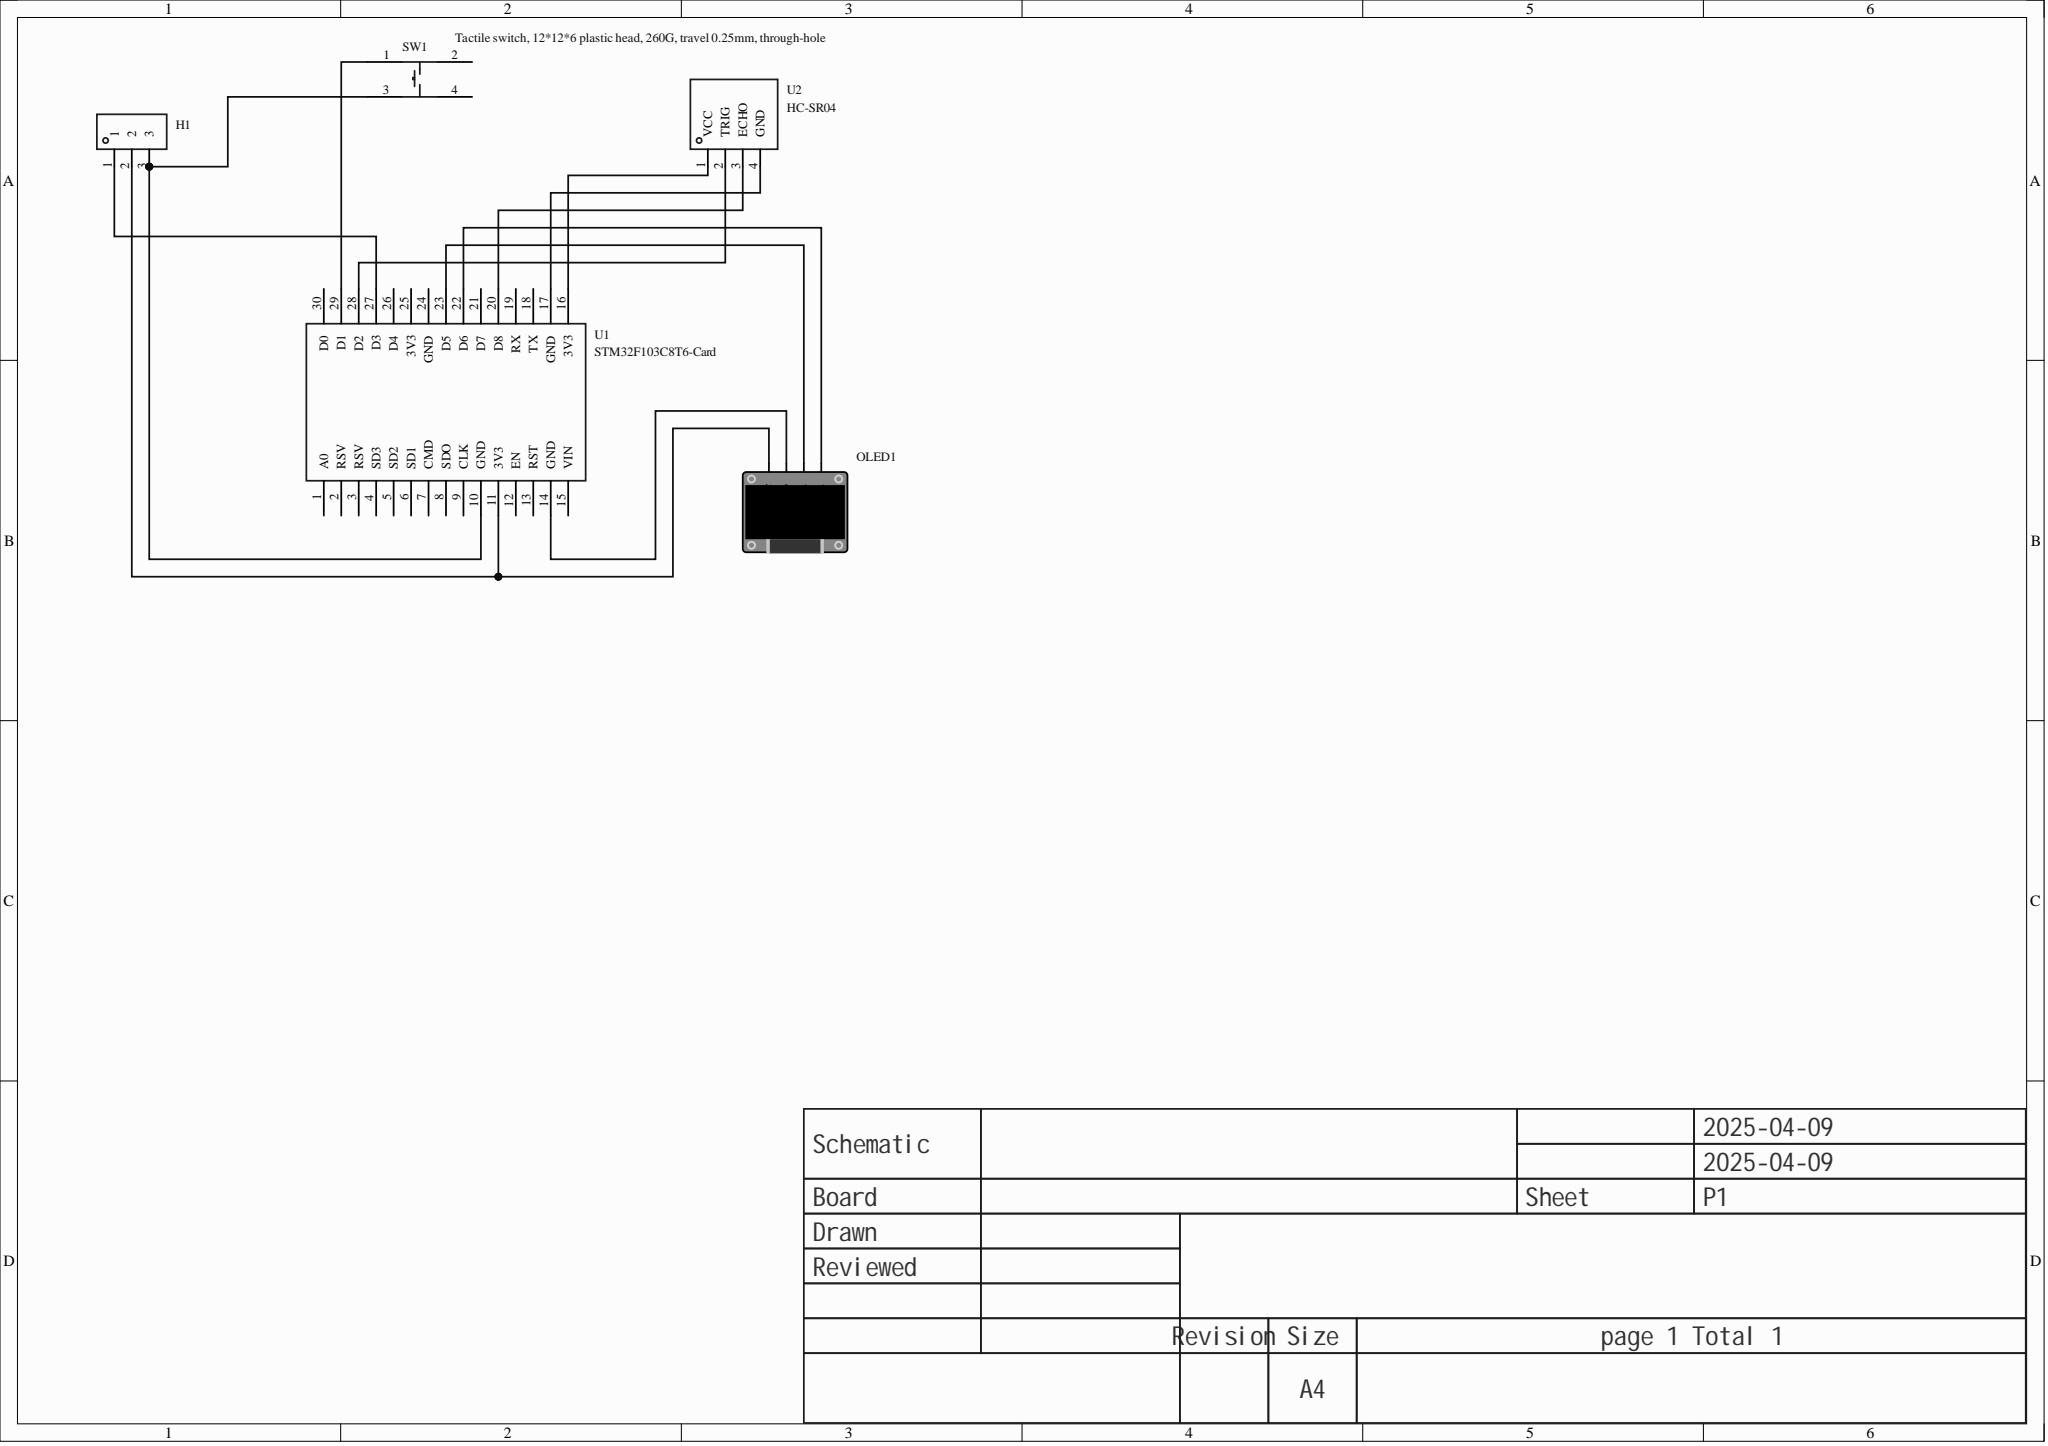Circuit board | Altium Designer | 5 parts | 11 nets
Bill of materials:
Comment,Description,Designator,Footprint,LibRef,Quantity
"","","H1","HDR-TH_3P-P2.54-V-F","HDR-F_2.54_1x3P","1"
"","","OLED1","0.96OLED_4P","0.96OLED模块_4P","1"
"Tactile switch, 12*12*6 plastic head, 260G, travel 0.25mm, through-hole","","SW1","KEY-TH_4P-L12.0-W12.0-P5.00-LS12.5","轻触开关,12*12*6塑头,260G,行程0.25mm,直插","1"
"STM32F103C8T6-Card","","U1","CONN-TH_L53.3-W22.9_STM32F103C8T6-CARD","STM32F103C8T6-Card","1"
"HC-SR04","","U2","TH_HC-SR04V","HC-SR04","1"
Netlist (Protel format):
[
H1
HDR-TH_3P-P2.54-V-F




]
[
OLED1
0.96OLED_4P




]
[
SW1
KEY-TH_4P-L12.0-W12.0-P5.00-LS12.5
Tactile switch, 12*12*6 plastic head, 260G, travel 0.25mm, through-hole



]
[
U1
CONN-TH_L53.3-W22.9_STM32F103C8T6-CARD
STM32F103C8T6-Card



]
[
U2
TH_HC-SR04V
HC-SR04



]
(
NetU1_28
U1-28
U2-2
)
(
NetU1_20
U1-20
U2-3
)
(
NetU1_17
U1-17
U2-4
)
(
NetU1_16
U1-16
U2-1
)
(
NetSW1_1
SW1-1
U1-29
)
(
NetOLED1_4
OLED1-4
U1-22
)
(
NetOLED1_3
OLED1-3
U1-23
)
(
NetOLED1_2
OLED1-2
U1-14
)
(
NetH1_3
H1-3
SW1-3
U1-10
)
(
NetH1_2
H1-2
OLED1-1
U1-11
)
(
NetH1_1
H1-1
U1-27
)